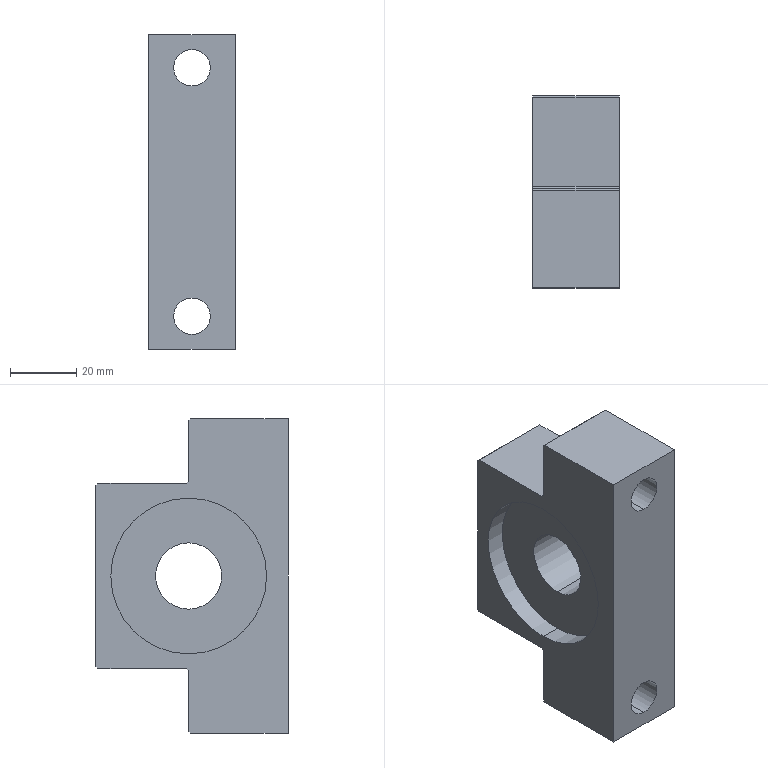Part | STEP file | 0244_Z_003_BUN20_1 | 1 solid | 31 faces | box 26 x 58 x 95 mm | volume 83295 mm3 | plane 19 | cylinder 12 | commonest cylinder face diameters 11 x4 47 x4 20 x2 49.5 x2